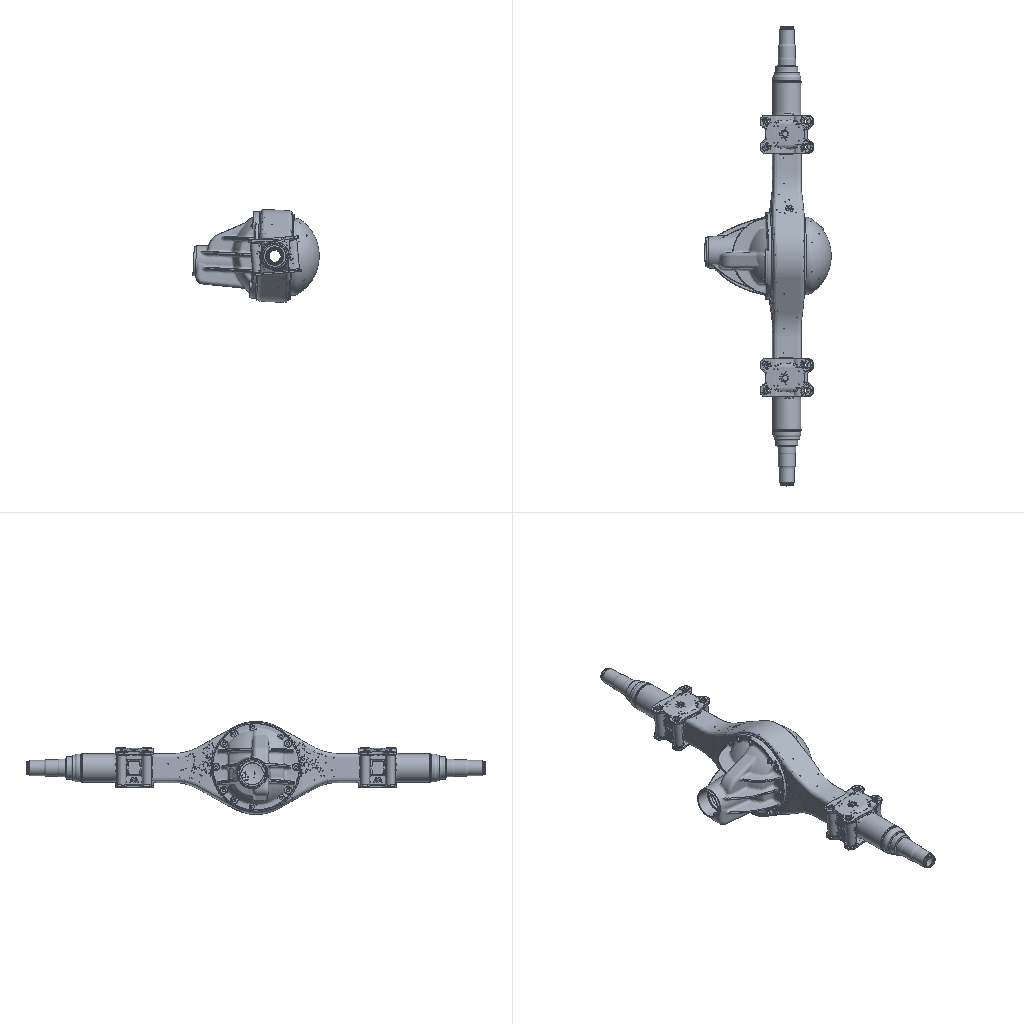Simulation study | nastran
Set-up summary:
category,name,step,type,value,unit,region
solver,nx_nastran
units,not stated in the deck,,not stated
analysis,deck,,static,static
analysis,solution,,SOL,101
load_step,SUBCASE 1,1,SUBCASE,SPC=1 LOAD=3
load_step,SUBCASE 2,2,SUBCASE,SPC=1 LOAD=4
load_step,requested,,,2
mesh,nodes,,,374598
mesh,elements,,,414074
element_type,CHEXA,,unverified,175736
element_type,CPENTA,,unverified,6788
element_type,CTETRA,,solid,414074
load,load commands in deck,,count,2
bc,support commands in deck,,count,2
check,setup vs results,,match,"every grid point's frame and coordinates and every element id; grid points of CHEXA, CPENTA, CTETRA elements"
Nastran input file, long lists of numbers shortened:
$$------------------------------------------------------------------------------$
$$                                                                              $
$$ NASTRAN Input Deck Generated by HyperMesh Version  :11.0.0.4                 $
$$ Generated using HyperMesh-Nastran Template Version : 11.0.0.47
$$                                                                              $
$$   Template:  general                                                         $
$$                                                                              $
$$------------------------------------------------------------------------------$
$$------------------------------------------------------------------------------$
$$                      Executive Control Cards                                 $
$$------------------------------------------------------------------------------$
SOL 101
CEND
$$------------------------------------------------------------------------------$
$$                      Case Control Cards                                      $
$$------------------------------------------------------------------------------$
$
$HMNAME LOADSTEP               1"Load_Full"
SUBCASE       1
  LABEL= Load_Full
  SPC =        1
  LOAD =        3
  DISPLACEMENT = ALL
  STRESS = ALL
$
$HMNAME LOADSTEP               2"Load_2.5g"
SUBCASE       2
  LABEL= Load_2.5g
  SPC =        1
  LOAD =        4
  DISPLACEMENT = ALL
  STRESS = ALL
$$------------------------------------------------------------------------------$
$$                      Bulk Data Cards                                         $
$$------------------------------------------------------------------------------$
BEGIN BULK
PARAM,AUTOSPC,YES
PARAM,POST,-1
$$
$$  GRID Data
$$
GRID          53        2759.983162.8658-227.241
GRID          54        2759.833162.8658-230.218
$ (374596 more lines like these left out)
$$
$$  SPOINT Data
$$
$$
$$------------------------------------------------------------------------------$
$$             Group Definitions                                                $
$$------------------------------------------------------------------------------$
$$
$$ RBE2 Elements - Multiple dependent nodes
$$
RBE2     3143432  891919  123456  666387  666389  666390  666395  666396+
+         666809  666817  666821  666823  666824  666828  666846  666872+
+         666873  666958  666962  667346  667347  667509  667559  667831+
+         667833  667834  667835  667837  667841  667844  668035  668057+
+         668347  668348  668349  668350  668354  668356  668358  668563+
+         668583  668603  668874  668875  668878  668879  668881  668884+
+         669070  669124  669125  669390  669397  669398  669399  669400+
+         669404  669882  669944  670005  670038  670061  670079  670091+
+         670126  670170  670215  670227  670376  670378  670386  670428+
+         670472  670490  670543
RBE2     3143433  891920  123456  663001  663002  663003  663004  663005+
+         663006  663007  663008  663009  663010  663011  663012  663013+
+         663014  663015  663016  663017  663018  663319  663346  663387+
+         663426  663427  663973  663977  663980  663981  663982  663985+
+         663987  663988  663991  663992  663995  663999  664000  664405+
+         664434  664474  664512  664513  665061  665062  665066  665067+
+         665068  665070  665073  665074  665075  665079  665081  665085+
+         665087  665491  665516  665560  665598  665599  666145  666149+
+         666152  666153  666154  666158  666159  666162  666163  666164+
+         666167  666171  666172
$ (2041 more lines like these left out)
$
$HMMOVE      399
$        3143432THRU     3143441 3580472THRU     3580473
$
$
$HMMOVE      408
$        3785584THRU     3785595
$
$
$  RBE3 Elements
$
RBE3     2819571          813047     123.0120261     123  354390.9879464+
+            123  3543892.7152-5     123  3804471.0-5        123  380444+
+       0.067626     123  290750.2660429     123  276040.5312839     123+
+         276030.1350475     123  290754
RBE3     2820914          814968  123456.1818618     123  777503.5357866+
+            123  777500.2107999     123  7775010.071552     123  777502
$ (11195 more lines like these left out)
$
$HMMOVE      399
$        2819571 2820914THRU     2820916 2820918THRU     2820920 2820922THRU
$        2820924 2820926THRU     2820928 2820938 2820942THRU     2820944 2820946
$ (452 more lines like these left out)
CHEXA     364054     141  354042  354043  354059  354058  379761  379762+
+         379778  379777
CHEXA     364055     141  354043  354044  354060  354059  379762  379763+
+         379779  379778
$ (351468 more lines like these left out)
$
$HMMOVE      141
$         364054THRU      364433  364435THRU      364489  364491THRU      364545
$         364547THRU      364601  364603THRU      364657  364659THRU      364826
$ (942 more lines like these left out)
CTETRA    800517     401  497524  566390  567071  497548
CTETRA    800518     401  546336  536057  517402  536070
$ (414072 more lines like these left out)
$
$  CPENTA Elements 6-noded
$
CPENTA    353881     141  343608  343610  343609  369214  369216  369215
CPENTA    353882     141  343611  343610  343679  369217  369216  369218
$ (6786 more lines like these left out)
$
$HMMOVE      401
$         800517THRU      801516  799517THRU      800516  798517THRU      799516
$         797517THRU      798516  796517THRU      797516  795517THRU      796516
$ (606 more lines like these left out)
PSOLID       401       1
$
$HMNAME PROP                 390"Seam" 5
$HWCOLOR PROP                390      53
PSOLID       390       5
$
$HMNAME PROP                 385"N620_Rear_Axle_385" 5
$HWCOLOR PROP                385      49
PSOLID       385       2
$
$HMNAME PROP                 384"N620_Rear_Axle_384" 5
$HWCOLOR PROP                384      62
PSOLID       384       2
$
$HMNAME PROP                 383"N620_Rear_Axle_383" 5
$HWCOLOR PROP                383      36
PSOLID       383       2
$
$HMNAME PROP                 382"N620_Rear_Axle_382" 5
$HWCOLOR PROP                382      21
PSOLID       382       2
$
$HMNAME PROP                 381"N620_Rear_Axle_381" 5
$HWCOLOR PROP                381      43
PSOLID       381       2
$
$HMNAME PROP                 358"N620_Rear_Axle_358" 5
$HWCOLOR PROP                358      37
PSOLID       358       4
$
$HMNAME PROP                 333"N620_Rear_Axle_333" 5
$HWCOLOR PROP                333      44
PSOLID       333       1
$
$HMNAME PROP                 320"N620_Rear_Axle_320" 5
$HWCOLOR PROP                320      52
PSOLID       320       4
$
$HMNAME PROP                 319"N620_Rear_Axle_319" 5
$HWCOLOR PROP                319      25
PSOLID       319       4
$
$HMNAME PROP                 318"N620_Rear_Axle_318" 5
$HWCOLOR PROP                318      44
PSOLID       318       4
$
$HMNAME PROP                 317"N620_Rear_Axle_317" 5
$HWCOLOR PROP                317      37
PSOLID       317       3
$
$HMNAME PROP                 155"N620_Rear_Axle_155" 5
$HWCOLOR PROP                155      49
PSOLID       155       2
$
$HMNAME PROP                 141"N620_Rear_Axle_141" 5
$HWCOLOR PROP                141      43
PSOLID       141       1
$$--------------------------------------------------------------
$$ HYPERMESH TAGS
$$--------------------------------------------------------------
$$BEGIN TAGS
$$END TAGS
$$
$$  MAT1 Data
$
$HMNAME MAT                    1"QT500" "MAT1"
$HWCOLOR MAT                   1       3
MAT1           1210000.0        0.28    7.8-9
$
$HMNAME MAT                    2"DL510" "MAT1"
$HWCOLOR MAT                   2      36
MAT1           2210000.0        0.28    7.8-9
$
$HMNAME MAT                    3"45#" "MAT1"
$HWCOLOR MAT                   3      36
MAT1           3210000.0        0.28    7.8-9
$
$HMNAME MAT                    4"Q235" "MAT1"
$HWCOLOR MAT                   4      36
MAT1           4210000.0        0.3     7.8-9
$
$HMNAME MAT                    5"weld" "MAT1"
$HWCOLOR MAT                   5      36
MAT1           5220000.0        0.28    7.8-9
$$
$$
$$
$$------------------------------------------------------------------------------$
$ (35 more lines like these left out)
LOAD           31.0        151.1       2
$
$HMNAME LOADCOL                4"Load_2.5g"
$HWCOLOR LOADCOL               4       6
$$
LOAD           41.0        377.7       2
$
$$
$$  SPC Data
$$
SPC            1 1042925  12356 0.0
SPC            1 1042924  1356  0.0
$
$$
$$  FORCE Data
$$
FORCE          2  891923       01.0     0.0     0.0     -100.0
FORCE          2  891928       01.0     0.0     0.0     -100.0
ENDDATA
Results summary:
result,analysis,,,static
result,last_loadstep,,,2
result,primary field,,,displacements
result,max displacement,,,3.807,model units